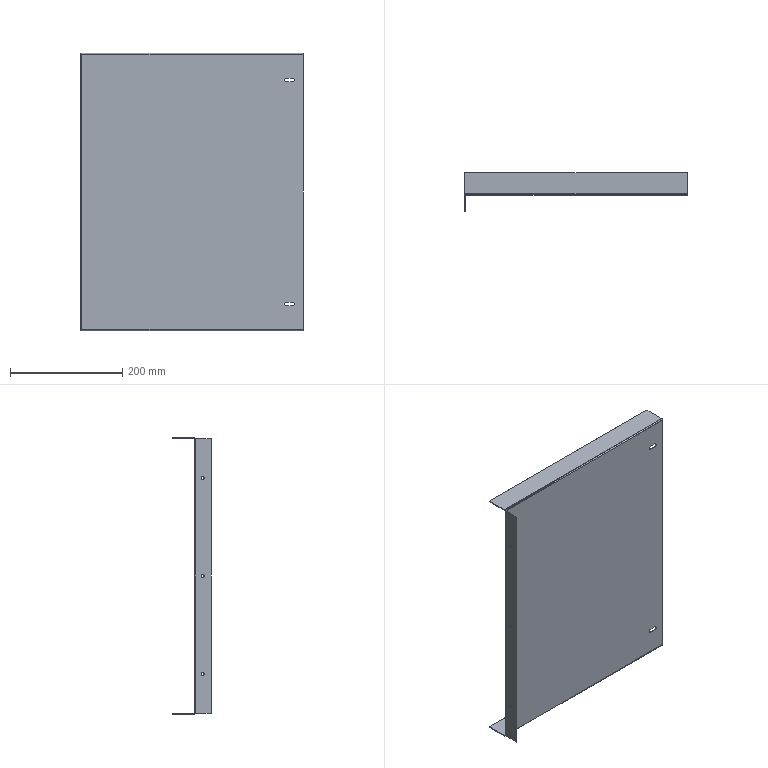Part | STEP file | PN_0047_protective cover_default_machined_ | 1 solid | 38 faces | box 398 x 68.5 x 495 mm | volume 360809 mm3 | plane 22 | cylinder 16 | commonest cylinder face diameters 5 x6 7 x4 1.473 x3 4.473 x3